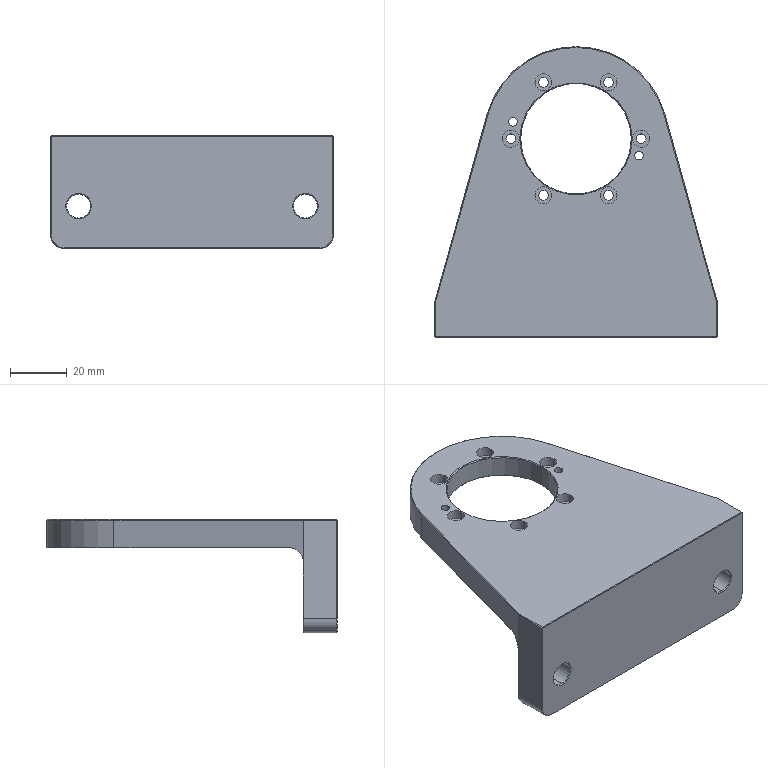NC program | NX | posted with a generic post | part box 100 x 102.5 x 40 mm
Lines 1 to 69 of 4503:
N10 G17 G21 G94 G90
(FLOOR_WALL_COPY , TOOL : D80)
N12 T19 M6
N14 G54
N16 G17 G0 G90 X-101.25 Y54.997 B0. C0. S6500 M3
N18 G43 Z30. H19
N20 Z3.
N22 G94 G1 Z0. F1500.
N24 X-96.25
N26 X96.25
N28 Y15.999
N30 X-96.25
N32 Y-23.
N34 X96.25
N36 X101.25
N38 Z3.
N40 G0 Z30.
N42 M5
(DRILLING_COPY_1 , TOOL : D6A45)
N44 T01 M6
N46 G54
N48 G17 G0 G90 X18.75 Y0. B0. C0. S5000 M3
N50 G43 Z30. H1
N52 G94 G81 G98 Z-1.6 F350. R3.
N54 X38.669 Y-11.5
N56 X18.75 Y-23.
N58 X12.797 Y-22.216
N60 X-1.169 Y-11.5
N62 Y11.5
N64 X18.75 Y23.
N66 X24.703 Y22.216
N68 X38.669 Y11.5
N70 G80
N72 G0 X38.669 Y11.5 Z30.
N74 M5
(DRILLING_COPY_1_COPY , TOOL : 2.8ZT)
N76 T16 M6
N78 G54
N80 G17 G0 G90 X24.703 Y22.216 B0. C0. S2000 M3
N82 G43 Z30. H16
N84 G94 G83 G98 Z-10.341 F150. Q2. R3.
N86 X12.797 Y-22.216
N88 G80
N90 G0 X12.797 Y-22.216 Z30.
N92 M5
(DRILLING_COPY_1_COPY_1 , TOOL : 3.4ZT)
N94 T03 M6
N96 G54
N98 G17 G0 G90 X18.75 Y23. B0. C0. S2000 M3
N100 G43 Z30. H3
N102 G94 G83 G98 Z-10.521 F180. Q2. R3.
N104 X-1.169 Y11.5
N106 Y-11.5
N108 X18.75 Y-23.
N110 X38.669 Y-11.5
N112 Y11.5
N114 G80
N116 G0 X38.669 Y11.5 Z30.
N118 M5